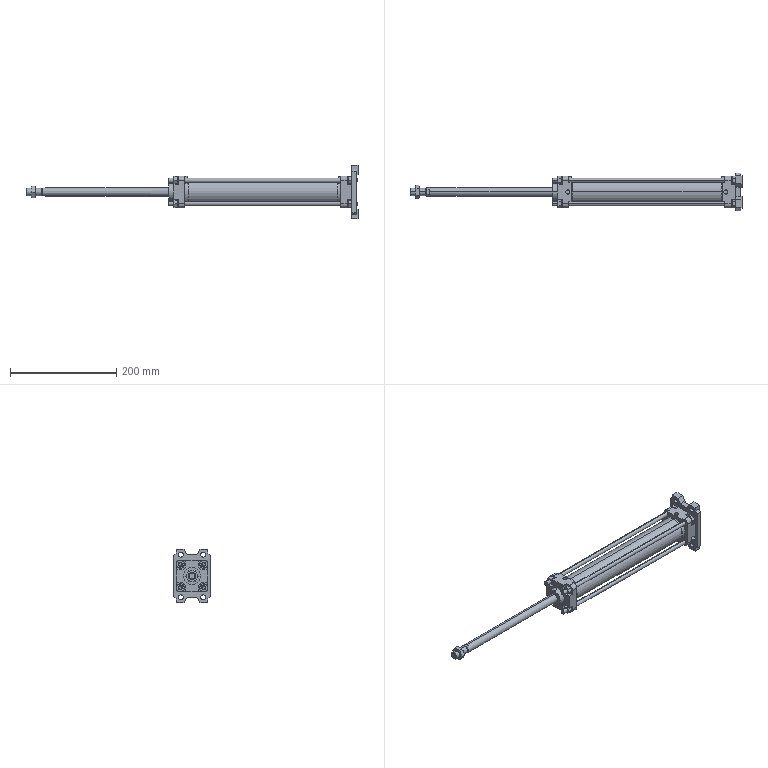Part | STEP file | CA2G40-250Z_0_0_0_ | 4 solids | 379 faces | box 624.042 x 71 x 100 mm | volume 473090 mm3 | plane 215 | cylinder 128 | cone 36 | commonest cylinder face diameters 8 x36 15.4 x24 21 x20 16 x12 9 x8 32 x6